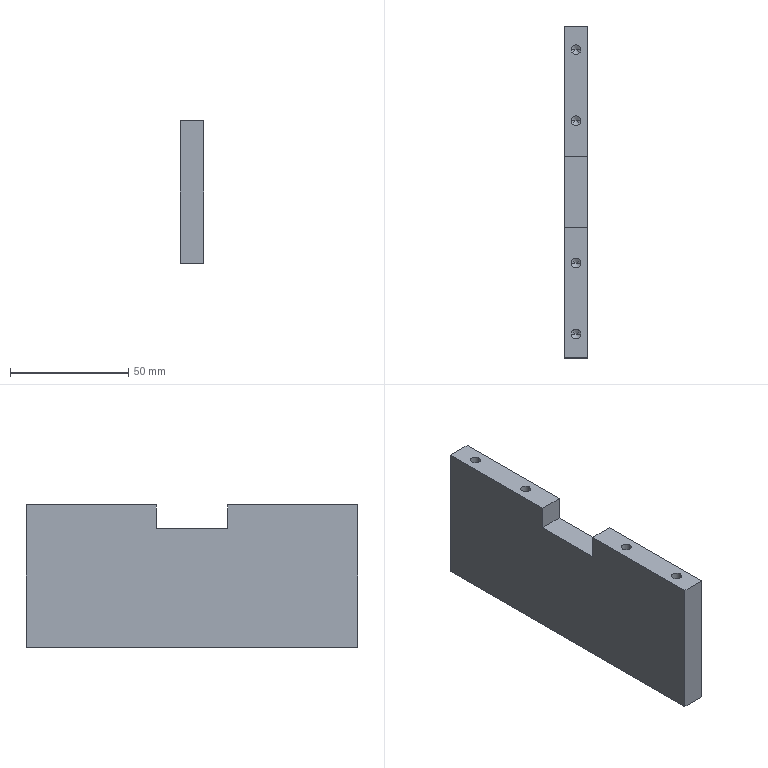Part | SolidWorks | features HoleWzd 2, Cut 1, Extrusion 1, LPattern 1 | 1 solid | 38 faces | box 10 x 140 x 60 mm | volume 79757 mm3 | cylinder 14 | cone 14 | plane 10 | commonest cylinder face diameters 4.2 x14
STEP:
#1=CARTESIAN_POINT('',(2.9,-60.,17.6));
#2=VERTEX_POINT('',#1);
#3=CARTESIAN_POINT('',(7.1,-60.,17.6));
#4=VERTEX_POINT('',#3);
#5=CARTESIAN_POINT('',(5.,-60.,17.6));
#6=DIRECTION('',(0.,0.,1.));
#7=DIRECTION('',(1.,0.,0.));
#8=AXIS2_PLACEMENT_3D('',#5,#6,#7);
#9=CIRCLE('',#8,2.1);
#10=EDGE_CURVE('',#2,#4,#9,.T.);
#11=ORIENTED_EDGE('',*,*,#10,.F.);
#12=CARTESIAN_POINT('',(2.9,-60.,30.));
#13=VERTEX_POINT('',#12);
#14=CARTESIAN_POINT('',(2.9,-60.,30.));
#15=DIRECTION('',(0.,0.,1.));
#16=VECTOR('',#15,1000.);
#17=LINE('',#14,#16);
#18=EDGE_CURVE('',#2,#13,#17,.T.);
#19=ORIENTED_EDGE('',*,*,#18,.T.);
#20=CARTESIAN_POINT('',(7.1,-60.,30.));
#21=VERTEX_POINT('',#20);
#22=CARTESIAN_POINT('',(5.,-60.,30.));
#23=DIRECTION('',(0.,0.,1.));
#24=DIRECTION('',(1.,0.,0.));
#25=AXIS2_PLACEMENT_3D('',#22,#23,#24);
#26=CIRCLE('',#25,2.1);
#27=EDGE_CURVE('',#13,#21,#26,.T.);
#28=ORIENTED_EDGE('',*,*,#27,.T.);
#29=CARTESIAN_POINT('',(7.1,-60.,30.));
#30=DIRECTION('',(0.,0.,1.));
#31=VECTOR('',#30,1000.);
#32=LINE('',#29,#31);
#33=EDGE_CURVE('',#4,#21,#32,.T.);
#34=ORIENTED_EDGE('',*,*,#33,.F.);
#35=EDGE_LOOP('',(#11,#19,#28,#34));
#36=FACE_OUTER_BOUND('',#35,.T.);
#37=CARTESIAN_POINT('',(5.,-60.,30.));
#38=DIRECTION('',(0.,0.,1.));
#39=DIRECTION('',(1.,0.,0.));
#40=AXIS2_PLACEMENT_3D('',#37,#38,#39);
#41=CYLINDRICAL_SURFACE('',#40,2.1);
#42=ADVANCED_FACE('',(#36),#41,.F.);
#43=CARTESIAN_POINT('',(5.,-60.,16.338));
#44=VERTEX_POINT('',#43);
#45=CARTESIAN_POINT('',(7.1,-60.,17.6));
#46=DIRECTION('',(0.8572,0.,0.515));
#47=VECTOR('',#46,1000.);
#48=LINE('',#45,#47);
#49=EDGE_CURVE('',#44,#4,#48,.T.);
#50=ORIENTED_EDGE('',*,*,#49,.F.);
#51=CARTESIAN_POINT('',(2.9,-60.,17.6));
#52=DIRECTION('',(-0.8572,0.,0.515));
#53=VECTOR('',#52,1000.);
#54=LINE('',#51,#53);
#55=EDGE_CURVE('',#44,#2,#54,.T.);
#56=ORIENTED_EDGE('',*,*,#55,.T.);
#57=ORIENTED_EDGE('',*,*,#10,.T.);
#58=EDGE_LOOP('',(#50,#56,#57));
#59=FACE_OUTER_BOUND('',#58,.T.);
#60=CARTESIAN_POINT('',(5.,-60.,17.6));
#61=DIRECTION('',(0.,0.,1.));
#62=DIRECTION('',(1.,0.,0.));
#63=AXIS2_PLACEMENT_3D('',#60,#61,#62);
#64=CONICAL_SURFACE('',#63,2.1,1.03);
#65=ADVANCED_FACE('',(#59),#64,.F.);
#66=CARTESIAN_POINT('',(2.9,-30.,17.6));
#67=VERTEX_POINT('',#66);
#68=CARTESIAN_POINT('',(7.1,-30.,17.6));
#69=VERTEX_POINT('',#68);
#70=CARTESIAN_POINT('',(5.,-30.,17.6));
#71=DIRECTION('',(0.,0.,1.));
#72=DIRECTION('',(1.,0.,0.));
#73=AXIS2_PLACEMENT_3D('',#70,#71,#72);
#74=CIRCLE('',#73,2.1);
#75=EDGE_CURVE('',#67,#69,#74,.T.);
#76=ORIENTED_EDGE('',*,*,#75,.F.);
#77=CARTESIAN_POINT('',(2.9,-30.,30.));
#78=VERTEX_POINT('',#77);
#79=CARTESIAN_POINT('',(2.9,-30.,30.));
#80=DIRECTION('',(0.,0.,1.));
#81=VECTOR('',#80,1000.);
#82=LINE('',#79,#81);
#83=EDGE_CURVE('',#67,#78,#82,.T.);
#84=ORIENTED_EDGE('',*,*,#83,.T.);
#85=CARTESIAN_POINT('',(7.1,-30.,30.));
#86=VERTEX_POINT('',#85);
#87=CARTESIAN_POINT('',(5.,-30.,30.));
#88=DIRECTION('',(0.,0.,1.));
#89=DIRECTION('',(1.,0.,0.));
#90=AXIS2_PLACEMENT_3D('',#87,#88,#89);
#91=CIRCLE('',#90,2.1);
#92=EDGE_CURVE('',#78,#86,#91,.T.);
#93=ORIENTED_EDGE('',*,*,#92,.T.);
#94=CARTESIAN_POINT('',(7.1,-30.,30.));
#95=DIRECTION('',(0.,0.,1.));
#96=VECTOR('',#95,1000.);
#97=LINE('',#94,#96);
#98=EDGE_CURVE('',#69,#86,#97,.T.);
#99=ORIENTED_EDGE('',*,*,#98,.F.);
#100=EDGE_LOOP('',(#76,#84,#93,#99));
#101=FACE_OUTER_BOUND('',#100,.T.);
#102=CARTESIAN_POINT('',(5.,-30.,30.));
#103=DIRECTION('',(0.,0.,1.));
#104=DIRECTION('',(1.,0.,0.));
#105=AXIS2_PLACEMENT_3D('',#102,#103,#104);
#106=CYLINDRICAL_SURFACE('',#105,2.1);
#107=ADVANCED_FACE('',(#101),#106,.F.);
#108=CARTESIAN_POINT('',(5.,-30.,16.338));
#109=VERTEX_POINT('',#108);
#110=CARTESIAN_POINT('',(7.1,-30.,17.6));
#111=DIRECTION('',(0.8572,0.,0.515));
#112=VECTOR('',#111,1000.);
#113=LINE('',#110,#112);
#114=EDGE_CURVE('',#109,#69,#113,.T.);
#115=ORIENTED_EDGE('',*,*,#114,.F.);
#116=CARTESIAN_POINT('',(2.9,-30.,17.6));
#117=DIRECTION('',(-0.8572,0.,0.515));
#118=VECTOR('',#117,1000.);
#119=LINE('',#116,#118);
#120=EDGE_CURVE('',#109,#67,#119,.T.);
#121=ORIENTED_EDGE('',*,*,#120,.T.);
#122=ORIENTED_EDGE('',*,*,#75,.T.);
#123=EDGE_LOOP('',(#115,#121,#122));
#124=FACE_OUTER_BOUND('',#123,.T.);
#125=CARTESIAN_POINT('',(5.,-30.,17.6));
#126=DIRECTION('',(0.,0.,1.));
#127=DIRECTION('',(1.,0.,0.));
#128=AXIS2_PLACEMENT_3D('',#125,#126,#127);
#129=CONICAL_SURFACE('',#128,2.1,1.03);
#130=ADVANCED_FACE('',(#124),#129,.F.);
#131=CARTESIAN_POINT('',(2.9,30.,17.6));
#132=VERTEX_POINT('',#131);
#133=CARTESIAN_POINT('',(7.1,30.,17.6));
#134=VERTEX_POINT('',#133);
#135=CARTESIAN_POINT('',(5.,30.,17.6));
#136=DIRECTION('',(0.,0.,1.));
#137=DIRECTION('',(1.,0.,0.));
#138=AXIS2_PLACEMENT_3D('',#135,#136,#137);
#139=CIRCLE('',#138,2.1);
#140=EDGE_CURVE('',#132,#134,#139,.T.);
#141=ORIENTED_EDGE('',*,*,#140,.F.);
#142=CARTESIAN_POINT('',(2.9,30.,30.));
#143=VERTEX_POINT('',#142);
#144=CARTESIAN_POINT('',(2.9,30.,30.));
#145=DIRECTION('',(0.,0.,1.));
#146=VECTOR('',#145,1000.);
#147=LINE('',#144,#146);
#148=EDGE_CURVE('',#132,#143,#147,.T.);
#149=ORIENTED_EDGE('',*,*,#148,.T.);
#150=CARTESIAN_POINT('',(7.1,30.,30.));
#151=VERTEX_POINT('',#150);
#152=CARTESIAN_POINT('',(5.,30.,30.));
#153=DIRECTION('',(0.,0.,1.));
#154=DIRECTION('',(1.,0.,0.));
#155=AXIS2_PLACEMENT_3D('',#152,#153,#154);
#156=CIRCLE('',#155,2.1);
#157=EDGE_CURVE('',#143,#151,#156,.T.);
#158=ORIENTED_EDGE('',*,*,#157,.T.);
#159=CARTESIAN_POINT('',(7.1,30.,30.));
#160=DIRECTION('',(0.,0.,1.));
#161=VECTOR('',#160,1000.);
#162=LINE('',#159,#161);
#163=EDGE_CURVE('',#134,#151,#162,.T.);
#164=ORIENTED_EDGE('',*,*,#163,.F.);
#165=EDGE_LOOP('',(#141,#149,#158,#164));
#166=FACE_OUTER_BOUND('',#165,.T.);
#167=CARTESIAN_POINT('',(5.,30.,30.));
#168=DIRECTION('',(0.,0.,1.));
#169=DIRECTION('',(1.,0.,0.));
#170=AXIS2_PLACEMENT_3D('',#167,#168,#169);
#171=CYLINDRICAL_SURFACE('',#170,2.1);
#172=ADVANCED_FACE('',(#166),#171,.F.);
#173=CARTESIAN_POINT('',(5.,30.,16.338));
#174=VERTEX_POINT('',#173);
#175=CARTESIAN_POINT('',(7.1,30.,17.6));
#176=DIRECTION('',(0.8572,0.,0.515));
#177=VECTOR('',#176,1000.);
#178=LINE('',#175,#177);
#179=EDGE_CURVE('',#174,#134,#178,.T.);
#180=ORIENTED_EDGE('',*,*,#179,.F.);
#181=CARTESIAN_POINT('',(2.9,30.,17.6));
#182=DIRECTION('',(-0.8572,0.,0.515));
#183=VECTOR('',#182,1000.);
#184=LINE('',#181,#183);
#185=EDGE_CURVE('',#174,#132,#184,.T.);
#186=ORIENTED_EDGE('',*,*,#185,.T.);
#187=ORIENTED_EDGE('',*,*,#140,.T.);
#188=EDGE_LOOP('',(#180,#186,#187));
#189=FACE_OUTER_BOUND('',#188,.T.);
#190=CARTESIAN_POINT('',(5.,30.,17.6));
#191=DIRECTION('',(0.,0.,1.));
#192=DIRECTION('',(1.,0.,0.));
#193=AXIS2_PLACEMENT_3D('',#190,#191,#192);
#194=CONICAL_SURFACE('',#193,2.1,1.03);
#195=ADVANCED_FACE('',(#189),#194,.F.);
#196=CARTESIAN_POINT('',(2.9,60.,17.6));
#197=VERTEX_POINT('',#196);
#198=CARTESIAN_POINT('',(7.1,60.,17.6));
#199=VERTEX_POINT('',#198);
#200=CARTESIAN_POINT('',(5.,60.,17.6));
#201=DIRECTION('',(0.,0.,1.));
#202=DIRECTION('',(1.,0.,0.));
#203=AXIS2_PLACEMENT_3D('',#200,#201,#202);
#204=CIRCLE('',#203,2.1);
#205=EDGE_CURVE('',#197,#199,#204,.T.);
#206=ORIENTED_EDGE('',*,*,#205,.F.);
#207=CARTESIAN_POINT('',(2.9,60.,30.));
#208=VERTEX_POINT('',#207);
#209=CARTESIAN_POINT('',(2.9,60.,30.));
#210=DIRECTION('',(0.,0.,1.));
#211=VECTOR('',#210,1000.);
#212=LINE('',#209,#211);
#213=EDGE_CURVE('',#197,#208,#212,.T.);
#214=ORIENTED_EDGE('',*,*,#213,.T.);
#215=CARTESIAN_POINT('',(7.1,60.,30.));
#216=VERTEX_POINT('',#215);
#217=CARTESIAN_POINT('',(5.,60.,30.));
#218=DIRECTION('',(0.,0.,1.));
#219=DIRECTION('',(1.,0.,0.));
#220=AXIS2_PLACEMENT_3D('',#217,#218,#219);
#221=CIRCLE('',#220,2.1);
#222=EDGE_CURVE('',#208,#216,#221,.T.);
#223=ORIENTED_EDGE('',*,*,#222,.T.);
#224=CARTESIAN_POINT('',(7.1,60.,30.));
#225=DIRECTION('',(0.,0.,1.));
#226=VECTOR('',#225,1000.);
#227=LINE('',#224,#226);
#228=EDGE_CURVE('',#199,#216,#227,.T.);
#229=ORIENTED_EDGE('',*,*,#228,.F.);
#230=EDGE_LOOP('',(#206,#214,#223,#229));
#231=FACE_OUTER_BOUND('',#230,.T.);
#232=CARTESIAN_POINT('',(5.,60.,30.));
#233=DIRECTION('',(0.,0.,1.));
#234=DIRECTION('',(1.,0.,0.));
#235=AXIS2_PLACEMENT_3D('',#232,#233,#234);
#236=CYLINDRICAL_SURFACE('',#235,2.1);
#237=ADVANCED_FACE('',(#231),#236,.F.);
#238=CARTESIAN_POINT('',(5.,60.,16.338));
#239=VERTEX_POINT('',#238);
#240=CARTESIAN_POINT('',(7.1,60.,17.6));
#241=DIRECTION('',(0.8572,0.,0.515));
#242=VECTOR('',#241,1000.);
#243=LINE('',#240,#242);
#244=EDGE_CURVE('',#239,#199,#243,.T.);
#245=ORIENTED_EDGE('',*,*,#244,.F.);
#246=CARTESIAN_POINT('',(2.9,60.,17.6));
#247=DIRECTION('',(-0.8572,0.,0.515));
#248=VECTOR('',#247,1000.);
#249=LINE('',#246,#248);
#250=EDGE_CURVE('',#239,#197,#249,.T.);
#251=ORIENTED_EDGE('',*,*,#250,.T.);
#252=ORIENTED_EDGE('',*,*,#205,.T.);
#253=EDGE_LOOP('',(#245,#251,#252));
#254=FACE_OUTER_BOUND('',#253,.T.);
#255=CARTESIAN_POINT('',(5.,60.,17.6));
#256=DIRECTION('',(0.,0.,1.));
#257=DIRECTION('',(1.,0.,0.));
#258=AXIS2_PLACEMENT_3D('',#255,#256,#257);
#259=CONICAL_SURFACE('',#258,2.1,1.03);
#260=ADVANCED_FACE('',(#254),#259,.F.);
#261=CARTESIAN_POINT('',(5.,-60.,-16.338));
#262=VERTEX_POINT('',#261);
#263=CARTESIAN_POINT('',(2.9,-60.,-17.6));
#264=VERTEX_POINT('',#263);
#265=CARTESIAN_POINT('',(2.9,-60.,-17.6));
#266=DIRECTION('',(-0.8572,0.,-0.515));
#267=VECTOR('',#266,1000.);
#268=LINE('',#265,#267);
#269=EDGE_CURVE('',#262,#264,#268,.T.);
#270=ORIENTED_EDGE('',*,*,#269,.F.);
#271=CARTESIAN_POINT('',(7.1,-60.,-17.6));
#272=VERTEX_POINT('',#271);
#273=CARTESIAN_POINT('',(7.1,-60.,-17.6));
#274=DIRECTION('',(0.8572,0.,-0.515));
#275=VECTOR('',#274,1000.);
#276=LINE('',#273,#275);
#277=EDGE_CURVE('',#262,#272,#276,.T.);
#278=ORIENTED_EDGE('',*,*,#277,.T.);
#279=CARTESIAN_POINT('',(5.,-60.,-17.6));
#280=DIRECTION('',(0.,0.,-1.));
#281=DIRECTION('',(-1.,0.,0.));
#282=AXIS2_PLACEMENT_3D('',#279,#280,#281);
#283=CIRCLE('',#282,2.1);
#284=EDGE_CURVE('',#272,#264,#283,.T.);
#285=ORIENTED_EDGE('',*,*,#284,.T.);
#286=EDGE_LOOP('',(#270,#278,#285));
#287=FACE_OUTER_BOUND('',#286,.T.);
#288=CARTESIAN_POINT('',(5.,-60.,-17.6));
#289=DIRECTION('',(0.,0.,-1.));
#290=DIRECTION('',(-1.,0.,0.));
#291=AXIS2_PLACEMENT_3D('',#288,#289,#290);
#292=CONICAL_SURFACE('',#291,2.1,1.03);
#293=ADVANCED_FACE('',(#287),#292,.F.);
#294=ORIENTED_EDGE('',*,*,#284,.F.);
#295=CARTESIAN_POINT('',(7.1,-60.,-30.));
#296=VERTEX_POINT('',#295);
#297=CARTESIAN_POINT('',(7.1,-60.,-30.));
#298=DIRECTION('',(0.,0.,-1.));
#299=VECTOR('',#298,1000.);
#300=LINE('',#297,#299);
#301=EDGE_CURVE('',#272,#296,#300,.T.);
#302=ORIENTED_EDGE('',*,*,#301,.T.);
#303=CARTESIAN_POINT('',(2.9,-60.,-30.));
#304=VERTEX_POINT('',#303);
#305=CARTESIAN_POINT('',(5.,-60.,-30.));
#306=DIRECTION('',(0.,0.,-1.));
#307=DIRECTION('',(-1.,0.,0.));
#308=AXIS2_PLACEMENT_3D('',#305,#306,#307);
#309=CIRCLE('',#308,2.1);
#310=EDGE_CURVE('',#296,#304,#309,.T.);
#311=ORIENTED_EDGE('',*,*,#310,.T.);
#312=CARTESIAN_POINT('',(2.9,-60.,-30.));
#313=DIRECTION('',(0.,0.,-1.));
#314=VECTOR('',#313,1000.);
#315=LINE('',#312,#314);
#316=EDGE_CURVE('',#264,#304,#315,.T.);
#317=ORIENTED_EDGE('',*,*,#316,.F.);
#318=EDGE_LOOP('',(#294,#302,#311,#317));
#319=FACE_OUTER_BOUND('',#318,.T.);
#320=CARTESIAN_POINT('',(5.,-60.,-30.));
#321=DIRECTION('',(0.,0.,-1.));
#322=DIRECTION('',(-1.,0.,0.));
#323=AXIS2_PLACEMENT_3D('',#320,#321,#322);
#324=CYLINDRICAL_SURFACE('',#323,2.1);
#325=ADVANCED_FACE('',(#319),#324,.F.);
#326=CARTESIAN_POINT('',(7.1,0.,-17.6));
#327=VERTEX_POINT('',#326);
#328=CARTESIAN_POINT('',(2.9,0.,-17.6));
#329=VERTEX_POINT('',#328);
#330=CARTESIAN_POINT('',(5.,0.,-17.6));
#331=DIRECTION('',(0.,0.,-1.));
#332=DIRECTION('',(-1.,0.,0.));
#333=AXIS2_PLACEMENT_3D('',#330,#331,#332);
#334=CIRCLE('',#333,2.1);
#335=EDGE_CURVE('',#327,#329,#334,.T.);
#336=ORIENTED_EDGE('',*,*,#335,.F.);
#337=CARTESIAN_POINT('',(7.1,0.,-30.));
#338=VERTEX_POINT('',#337);
#339=CARTESIAN_POINT('',(7.1,0.,-30.));
#340=DIRECTION('',(0.,0.,-1.));
#341=VECTOR('',#340,1000.);
#342=LINE('',#339,#341);
#343=EDGE_CURVE('',#327,#338,#342,.T.);
#344=ORIENTED_EDGE('',*,*,#343,.T.);
#345=CARTESIAN_POINT('',(2.9,0.,-30.));
#346=VERTEX_POINT('',#345);
#347=CARTESIAN_POINT('',(5.,0.,-30.));
#348=DIRECTION('',(0.,0.,-1.));
#349=DIRECTION('',(-1.,0.,0.));
#350=AXIS2_PLACEMENT_3D('',#347,#348,#349);
#351=CIRCLE('',#350,2.1);
#352=EDGE_CURVE('',#338,#346,#351,.T.);
#353=ORIENTED_EDGE('',*,*,#352,.T.);
#354=CARTESIAN_POINT('',(2.9,0.,-30.));
#355=DIRECTION('',(0.,0.,-1.));
#356=VECTOR('',#355,1000.);
#357=LINE('',#354,#356);
#358=EDGE_CURVE('',#329,#346,#357,.T.);
#359=ORIENTED_EDGE('',*,*,#358,.F.);
#360=EDGE_LOOP('',(#336,#344,#353,#359));
#361=FACE_OUTER_BOUND('',#360,.T.);
#362=CARTESIAN_POINT('',(5.,0.,-30.));
#363=DIRECTION('',(0.,0.,-1.));
#364=DIRECTION('',(-1.,0.,0.));
#365=AXIS2_PLACEMENT_3D('',#362,#363,#364);
#366=CYLINDRICAL_SURFACE('',#365,2.1);
#367=ADVANCED_FACE('',(#361),#366,.F.);
#368=CARTESIAN_POINT('',(5.,0.,-16.338));
#369=VERTEX_POINT('',#368);
#370=CARTESIAN_POINT('',(2.9,0.,-17.6));
#371=DIRECTION('',(-0.8572,0.,-0.515));
#372=VECTOR('',#371,1000.);
#373=LINE('',#370,#372);
#374=EDGE_CURVE('',#369,#329,#373,.T.);
#375=ORIENTED_EDGE('',*,*,#374,.F.);
#376=CARTESIAN_POINT('',(7.1,0.,-17.6));
#377=DIRECTION('',(0.8572,0.,-0.515));
#378=VECTOR('',#377,1000.);
#379=LINE('',#376,#378);
#380=EDGE_CURVE('',#369,#327,#379,.T.);
#381=ORIENTED_EDGE('',*,*,#380,.T.);
#382=ORIENTED_EDGE('',*,*,#335,.T.);
#383=EDGE_LOOP('',(#375,#381,#382));
#384=FACE_OUTER_BOUND('',#383,.T.);
#385=CARTESIAN_POINT('',(5.,0.,-17.6));
#386=DIRECTION('',(0.,0.,-1.));
#387=DIRECTION('',(-1.,0.,0.));
#388=AXIS2_PLACEMENT_3D('',#385,#386,#387);
#389=CONICAL_SURFACE('',#388,2.1,1.03);
#390=ADVANCED_FACE('',(#384),#389,.F.);
#391=CARTESIAN_POINT('',(7.1,60.,-17.6));
#392=VERTEX_POINT('',#391);
#393=CARTESIAN_POINT('',(2.9,60.,-17.6));
#394=VERTEX_POINT('',#393);
#395=CARTESIAN_POINT('',(5.,60.,-17.6));
#396=DIRECTION('',(0.,0.,-1.));
#397=DIRECTION('',(-1.,0.,0.));
#398=AXIS2_PLACEMENT_3D('',#395,#396,#397);
#399=CIRCLE('',#398,2.1);
#400=EDGE_CURVE('',#392,#394,#399,.T.);
#401=ORIENTED_EDGE('',*,*,#400,.F.);
#402=CARTESIAN_POINT('',(7.1,60.,-30.));
#403=VERTEX_POINT('',#402);
#404=CARTESIAN_POINT('',(7.1,60.,-30.));
#405=DIRECTION('',(0.,0.,-1.));
#406=VECTOR('',#405,1000.);
#407=LINE('',#404,#406);
#408=EDGE_CURVE('',#392,#403,#407,.T.);
#409=ORIENTED_EDGE('',*,*,#408,.T.);
#410=CARTESIAN_POINT('',(2.9,60.,-30.));
#411=VERTEX_POINT('',#410);
#412=CARTESIAN_POINT('',(5.,60.,-30.));
#413=DIRECTION('',(0.,0.,-1.));
#414=DIRECTION('',(-1.,0.,0.));
#415=AXIS2_PLACEMENT_3D('',#412,#413,#414);
#416=CIRCLE('',#415,2.1);
#417=EDGE_CURVE('',#403,#411,#416,.T.);
#418=ORIENTED_EDGE('',*,*,#417,.T.);
#419=CARTESIAN_POINT('',(2.9,60.,-30.));
#420=DIRECTION('',(0.,0.,-1.));
#421=VECTOR('',#420,1000.);
#422=LINE('',#419,#421);
#423=EDGE_CURVE('',#394,#411,#422,.T.);
#424=ORIENTED_EDGE('',*,*,#423,.F.);
#425=EDGE_LOOP('',(#401,#409,#418,#424));
#426=FACE_OUTER_BOUND('',#425,.T.);
#427=CARTESIAN_POINT('',(5.,60.,-30.));
#428=DIRECTION('',(0.,0.,-1.));
#429=DIRECTION('',(-1.,0.,0.));
#430=AXIS2_PLACEMENT_3D('',#427,#428,#429);
#431=CYLINDRICAL_SURFACE('',#430,2.1);
#432=ADVANCED_FACE('',(#426),#431,.F.);
#433=CARTESIAN_POINT('',(5.,60.,-16.338));
#434=VERTEX_POINT('',#433);
#435=CARTESIAN_POINT('',(2.9,60.,-17.6));
#436=DIRECTION('',(-0.8572,0.,-0.515));
#437=VECTOR('',#436,1000.);
#438=LINE('',#435,#437);
#439=EDGE_CURVE('',#434,#394,#438,.T.);
#440=ORIENTED_EDGE('',*,*,#439,.F.);
#441=CARTESIAN_POINT('',(7.1,60.,-17.6));
#442=DIRECTION('',(0.8572,0.,-0.515));
#443=VECTOR('',#442,1000.);
#444=LINE('',#441,#443);
#445=EDGE_CURVE('',#434,#392,#444,.T.);
#446=ORIENTED_EDGE('',*,*,#445,.T.);
#447=ORIENTED_EDGE('',*,*,#400,.T.);
#448=EDGE_LOOP('',(#440,#446,#447));
#449=FACE_OUTER_BOUND('',#448,.T.);
#450=CARTESIAN_POINT('',(5.,60.,-17.6));
#451=DIRECTION('',(0.,0.,-1.));
#452=DIRECTION('',(-1.,0.,0.));
#453=AXIS2_PLACEMENT_3D('',#450,#451,#452);
#454=CONICAL_SURFACE('',#453,2.1,1.03);
#455=ADVANCED_FACE('',(#449),#454,.F.);
#456=CARTESIAN_POINT('',(5.,-60.,30.));
#457=DIRECTION('',(0.,0.,1.));
#458=DIRECTION('',(1.,0.,0.));
#459=AXIS2_PLACEMENT_3D('',#456,#457,#458);
#460=CIRCLE('',#459,2.1);
#461=EDGE_CURVE('',#21,#13,#460,.T.);
#462=ORIENTED_EDGE('',*,*,#461,.F.);
#463=ORIENTED_EDGE('',*,*,#27,.F.);
#464=EDGE_LOOP('',(#462,#463));
#465=FACE_BOUND('',#464,.T.);
#466=CARTESIAN_POINT('',(5.,-30.,30.));
#467=DIRECTION('',(0.,0.,1.));
#468=DIRECTION('',(1.,0.,0.));
#469=AXIS2_PLACEMENT_3D('',#466,#467,#468);
#470=CIRCLE('',#469,2.1);
#471=EDGE_CURVE('',#86,#78,#470,.T.);
#472=ORIENTED_EDGE('',*,*,#471,.F.);
#473=ORIENTED_EDGE('',*,*,#92,.F.);
#474=EDGE_LOOP('',(#472,#473));
#475=FACE_BOUND('',#474,.T.);
#476=CARTESIAN_POINT('',(10.,-15.,30.));
#477=VERTEX_POINT('',#476);
#478=CARTESIAN_POINT('',(10.,-70.,30.));
#479=VERTEX_POINT('',#478);
#480=CARTESIAN_POINT('',(10.,-70.,30.));
#481=DIRECTION('',(0.,-1.,0.));
#482=VECTOR('',#481,1000.);
#483=LINE('',#480,#482);
#484=EDGE_CURVE('',#477,#479,#483,.T.);
#485=ORIENTED_EDGE('',*,*,#484,.F.);
#486=CARTESIAN_POINT('',(0.,-15.,30.));
#487=VERTEX_POINT('',#486);
#488=CARTESIAN_POINT('',(10.,-15.,30.));
#489=DIRECTION('',(-1.,0.,0.));
#490=VECTOR('',#489,1000.);
#491=LINE('',#488,#490);
#492=EDGE_CURVE('',#477,#487,#491,.T.);
#493=ORIENTED_EDGE('',*,*,#492,.T.);
#494=CARTESIAN_POINT('',(0.,-70.,30.));
#495=VERTEX_POINT('',#494);
#496=CARTESIAN_POINT('',(0.,-70.,30.));
#497=DIRECTION('',(0.,-1.,0.));
#498=VECTOR('',#497,1000.);
#499=LINE('',#496,#498);
#500=EDGE_CURVE('',#487,#495,#499,.T.);
#501=ORIENTED_EDGE('',*,*,#500,.T.);
#502=CARTESIAN_POINT('',(10.,-70.,30.));
#503=DIRECTION('',(-1.,0.,0.));
#504=VECTOR('',#503,1000.);
#505=LINE('',#502,#504);
#506=EDGE_CURVE('',#479,#495,#505,.T.);
#507=ORIENTED_EDGE('',*,*,#506,.F.);
#508=EDGE_LOOP('',(#485,#493,#501,#507));
#509=FACE_OUTER_BOUND('',#508,.T.);
#510=CARTESIAN_POINT('',(10.,-70.,30.));
#511=DIRECTION('',(0.,0.,-1.));
#512=DIRECTION('',(-1.,0.,0.));
#513=AXIS2_PLACEMENT_3D('',#510,#511,#512);
#514=PLANE('',#513);
#515=ADVANCED_FACE('',(#465,#475,#509),#514,.F.);
#516=CARTESIAN_POINT('',(5.,0.,-30.));
#517=DIRECTION('',(0.,0.,-1.));
#518=DIRECTION('',(-1.,0.,0.));
#519=AXIS2_PLACEMENT_3D('',#516,#517,#518);
#520=CIRCLE('',#519,2.1);
#521=EDGE_CURVE('',#346,#338,#520,.T.);
#522=ORIENTED_EDGE('',*,*,#521,.F.);
#523=ORIENTED_EDGE('',*,*,#352,.F.);
#524=EDGE_LOOP('',(#522,#523));
#525=FACE_BOUND('',#524,.T.);
#526=CARTESIAN_POINT('',(5.,60.,-30.));
#527=DIRECTION('',(0.,0.,-1.));
#528=DIRECTION('',(-1.,0.,0.));
#529=AXIS2_PLACEMENT_3D('',#526,#527,#528);
#530=CIRCLE('',#529,2.1);
#531=EDGE_CURVE('',#411,#403,#530,.T.);
#532=ORIENTED_EDGE('',*,*,#531,.F.);
#533=ORIENTED_EDGE('',*,*,#417,.F.);
#534=EDGE_LOOP('',(#532,#533));
#535=FACE_BOUND('',#534,.T.);
#536=CARTESIAN_POINT('',(0.,-70.,-30.));
#537=VERTEX_POINT('',#536);
#538=CARTESIAN_POINT('',(0.,70.,-30.));
#539=VERTEX_POINT('',#538);
#540=CARTESIAN_POINT('',(0.,-70.,-30.));
#541=DIRECTION('',(0.,1.,0.));
#542=VECTOR('',#541,1000.);
#543=LINE('',#540,#542);
#544=EDGE_CURVE('',#537,#539,#543,.T.);
#545=ORIENTED_EDGE('',*,*,#544,.T.);
#546=CARTESIAN_POINT('',(10.,70.,-30.));
#547=VERTEX_POINT('',#546);
#548=CARTESIAN_POINT('',(10.,70.,-30.));
#549=DIRECTION('',(-1.,0.,0.));
#550=VECTOR('',#549,1000.);
#551=LINE('',#548,#550);
#552=EDGE_CURVE('',#547,#539,#551,.T.);
#553=ORIENTED_EDGE('',*,*,#552,.F.);
#554=CARTESIAN_POINT('',(10.,-70.,-30.));
#555=VERTEX_POINT('',#554);
#556=CARTESIAN_POINT('',(10.,-70.,-30.));
#557=DIRECTION('',(0.,1.,0.));
#558=VECTOR('',#557,1000.);
#559=LINE('',#556,#558);
#560=EDGE_CURVE('',#555,#547,#559,.T.);
#561=ORIENTED_EDGE('',*,*,#560,.F.);
#562=CARTESIAN_POINT('',(10.,-70.,-30.));
#563=DIRECTION('',(-1.,0.,0.));
#564=VECTOR('',#563,1000.);
#565=LINE('',#562,#564);
#566=EDGE_CURVE('',#555,#537,#565,.T.);
#567=ORIENTED_EDGE('',*,*,#566,.T.);
#568=EDGE_LOOP('',(#545,#553,#561,#567));
#569=FACE_OUTER_BOUND('',#568,.T.);
#570=CARTESIAN_POINT('',(5.,-60.,-30.));
#571=DIRECTION('',(0.,0.,-1.));
#572=DIRECTION('',(-1.,0.,0.));
#573=AXIS2_PLACEMENT_3D('',#570,#571,#572);
#574=CIRCLE('',#573,2.1);
#575=EDGE_CURVE('',#304,#296,#574,.T.);
#576=ORIENTED_EDGE('',*,*,#575,.F.);
#577=ORIENTED_EDGE('',*,*,#310,.F.);
#578=EDGE_LOOP('',(#576,#577));
#579=FACE_BOUND('',#578,.T.);
#580=CARTESIAN_POINT('',(10.,-70.,-30.));
#581=DIRECTION('',(0.,0.,1.));
#582=DIRECTION('',(1.,0.,0.));
#583=AXIS2_PLACEMENT_3D('',#580,#581,#582);
#584=PLANE('',#583);
#585=ADVANCED_FACE('',(#525,#535,#569,#579),#584,.F.);
#586=CARTESIAN_POINT('',(0.,70.,30.));
#587=VERTEX_POINT('',#586);
#588=CARTESIAN_POINT('',(0.,70.,30.));
#589=DIRECTION('',(0.,0.,1.));
#590=VECTOR('',#589,1000.);
#591=LINE('',#588,#590);
#592=EDGE_CURVE('',#539,#587,#591,.T.);
#593=ORIENTED_EDGE('',*,*,#592,.T.);
#594=CARTESIAN_POINT('',(10.,70.,30.));
#595=VERTEX_POINT('',#594);
#596=CARTESIAN_POINT('',(10.,70.,30.));
#597=DIRECTION('',(-1.,0.,0.));
#598=VECTOR('',#597,1000.);
#599=LINE('',#596,#598);
#600=EDGE_CURVE('',#595,#587,#599,.T.);
#601=ORIENTED_EDGE('',*,*,#600,.F.);
#602=CARTESIAN_POINT('',(10.,70.,30.));
#603=DIRECTION('',(0.,0.,1.));
#604=VECTOR('',#603,1000.);
#605=LINE('',#602,#604);
#606=EDGE_CURVE('',#547,#595,#605,.T.);
#607=ORIENTED_EDGE('',*,*,#606,.F.);
#608=ORIENTED_EDGE('',*,*,#552,.T.);
#609=EDGE_LOOP('',(#593,#601,#607,#608));
#610=FACE_OUTER_BOUND('',#609,.T.);
#611=CARTESIAN_POINT('',(10.,70.,30.));
#612=DIRECTION('',(0.,-1.,0.));
#613=DIRECTION('',(0.,0.,-1.));
#614=AXIS2_PLACEMENT_3D('',#611,#612,#613);
#615=PLANE('',#614);
#616=ADVANCED_FACE('',(#610),#615,.F.);
#617=CARTESIAN_POINT('',(5.,30.,30.));
#618=DIRECTION('',(0.,0.,1.));
#619=DIRECTION('',(1.,0.,0.));
#620=AXIS2_PLACEMENT_3D('',#617,#618,#619);
#621=CIRCLE('',#620,2.1);
#622=EDGE_CURVE('',#151,#143,#621,.T.);
#623=ORIENTED_EDGE('',*,*,#622,.F.);
#624=ORIENTED_EDGE('',*,*,#157,.F.);
#625=EDGE_LOOP('',(#623,#624));
#626=FACE_BOUND('',#625,.T.);
#627=CARTESIAN_POINT('',(5.,60.,30.));
#628=DIRECTION('',(0.,0.,1.));
#629=DIRECTION('',(1.,0.,0.));
#630=AXIS2_PLACEMENT_3D('',#627,#628,#629);
#631=CIRCLE('',#630,2.1);
#632=EDGE_CURVE('',#216,#208,#631,.T.);
#633=ORIENTED_EDGE('',*,*,#632,.F.);
#634=ORIENTED_EDGE('',*,*,#222,.F.);
#635=EDGE_LOOP('',(#633,#634));
#636=FACE_BOUND('',#635,.T.);
#637=CARTESIAN_POINT('',(0.,15.,30.));
#638=VERTEX_POINT('',#637);
#639=CARTESIAN_POINT('',(0.,-70.,30.));
#640=DIRECTION('',(0.,-1.,0.));
#641=VECTOR('',#640,1000.);
#642=LINE('',#639,#641);
#643=EDGE_CURVE('',#587,#638,#642,.T.);
#644=ORIENTED_EDGE('',*,*,#643,.T.);
#645=CARTESIAN_POINT('',(10.,15.,30.));
#646=VERTEX_POINT('',#645);
#647=CARTESIAN_POINT('',(10.,15.,30.));
#648=DIRECTION('',(-1.,0.,0.));
#649=VECTOR('',#648,1000.);
#650=LINE('',#647,#649);
#651=EDGE_CURVE('',#646,#638,#650,.T.);
#652=ORIENTED_EDGE('',*,*,#651,.F.);
#653=CARTESIAN_POINT('',(10.,-70.,30.));
#654=DIRECTION('',(0.,-1.,0.));
#655=VECTOR('',#654,1000.);
#656=LINE('',#653,#655);
#657=EDGE_CURVE('',#595,#646,#656,.T.);
#658=ORIENTED_EDGE('',*,*,#657,.F.);
#659=ORIENTED_EDGE('',*,*,#600,.T.);
#660=EDGE_LOOP('',(#644,#652,#658,#659));
#661=FACE_OUTER_BOUND('',#660,.T.);
#662=CARTESIAN_POINT('',(10.,-70.,30.));
#663=DIRECTION('',(0.,0.,-1.));
#664=DIRECTION('',(-1.,0.,0.));
#665=AXIS2_PLACEMENT_3D('',#662,#663,#664);
#666=PLANE('',#665);
#667=ADVANCED_FACE('',(#626,#636,#661),#666,.F.);
#668=CARTESIAN_POINT('',(0.,-70.,30.));
#669=DIRECTION('',(0.,0.,-1.));
#670=VECTOR('',#669,1000.);
#671=LINE('',#668,#670);
#672=EDGE_CURVE('',#495,#537,#671,.T.);
#673=ORIENTED_EDGE('',*,*,#672,.T.);
#674=ORIENTED_EDGE('',*,*,#566,.F.);
#675=CARTESIAN_POINT('',(10.,-70.,30.));
#676=DIRECTION('',(0.,0.,-1.));
#677=VECTOR('',#676,1000.);
#678=LINE('',#675,#677);
#679=EDGE_CURVE('',#479,#555,#678,.T.);
#680=ORIENTED_EDGE('',*,*,#679,.F.);
#681=ORIENTED_EDGE('',*,*,#506,.T.);
#682=EDGE_LOOP('',(#673,#674,#680,#681));
#683=FACE_OUTER_BOUND('',#682,.T.);
#684=CARTESIAN_POINT('',(10.,-70.,30.));
#685=DIRECTION('',(0.,1.,0.));
#686=DIRECTION('',(0.,0.,1.));
#687=AXIS2_PLACEMENT_3D('',#684,#685,#686);
#688=PLANE('',#687);
#689=ADVANCED_FACE('',(#683),#688,.F.);
#690=CARTESIAN_POINT('',(10.,15.,20.));
#691=VERTEX_POINT('',#690);
#692=CARTESIAN_POINT('',(10.,-15.,20.));
#693=VERTEX_POINT('',#692);
#694=CARTESIAN_POINT('',(10.,-15.,20.));
#695=DIRECTION('',(0.,-1.,0.));
#696=VECTOR('',#695,1000.);
#697=LINE('',#694,#696);
#698=EDGE_CURVE('',#691,#693,#697,.T.);
#699=ORIENTED_EDGE('',*,*,#698,.T.);
#700=CARTESIAN_POINT('',(10.,-15.,30.));
#701=DIRECTION('',(0.,0.,1.));
#702=VECTOR('',#701,1000.);
#703=LINE('',#700,#702);
#704=EDGE_CURVE('',#693,#477,#703,.T.);
#705=ORIENTED_EDGE('',*,*,#704,.T.);
#706=ORIENTED_EDGE('',*,*,#484,.T.);
#707=ORIENTED_EDGE('',*,*,#679,.T.);
#708=ORIENTED_EDGE('',*,*,#560,.T.);
#709=ORIENTED_EDGE('',*,*,#606,.T.);
#710=ORIENTED_EDGE('',*,*,#657,.T.);
#711=CARTESIAN_POINT('',(10.,15.,30.));
#712=DIRECTION('',(0.,0.,-1.));
#713=VECTOR('',#712,1000.);
#714=LINE('',#711,#713);
#715=EDGE_CURVE('',#646,#691,#714,.T.);
#716=ORIENTED_EDGE('',*,*,#715,.T.);
#717=EDGE_LOOP('',(#699,#705,#706,#707,#708,#709,#710,#716));
#718=FACE_OUTER_BOUND('',#717,.T.);
#719=CARTESIAN_POINT('',(10.,70.,-30.));
#720=DIRECTION('',(-1.,0.,0.));
#721=DIRECTION('',(0.,0.,1.));
#722=AXIS2_PLACEMENT_3D('',#719,#720,#721);
#723=PLANE('',#722);
#724=ADVANCED_FACE('',(#718),#723,.F.);
#725=CARTESIAN_POINT('',(0.,-15.,20.));
#726=VERTEX_POINT('',#725);
#727=CARTESIAN_POINT('',(0.,-15.,30.));
#728=DIRECTION('',(0.,0.,1.));
#729=VECTOR('',#728,1000.);
#730=LINE('',#727,#729);
#731=EDGE_CURVE('',#726,#487,#730,.T.);
#732=ORIENTED_EDGE('',*,*,#731,.F.);
#733=CARTESIAN_POINT('',(0.,15.,20.));
#734=VERTEX_POINT('',#733);
#735=CARTESIAN_POINT('',(0.,-15.,20.));
#736=DIRECTION('',(0.,-1.,0.));
#737=VECTOR('',#736,1000.);
#738=LINE('',#735,#737);
#739=EDGE_CURVE('',#734,#726,#738,.T.);
#740=ORIENTED_EDGE('',*,*,#739,.F.);
#741=CARTESIAN_POINT('',(0.,15.,30.));
#742=DIRECTION('',(0.,0.,-1.));
#743=VECTOR('',#742,1000.);
#744=LINE('',#741,#743);
#745=EDGE_CURVE('',#638,#734,#744,.T.);
#746=ORIENTED_EDGE('',*,*,#745,.F.);
#747=ORIENTED_EDGE('',*,*,#643,.F.);
#748=ORIENTED_EDGE('',*,*,#592,.F.);
#749=ORIENTED_EDGE('',*,*,#544,.F.);
#750=ORIENTED_EDGE('',*,*,#672,.F.);
#751=ORIENTED_EDGE('',*,*,#500,.F.);
#752=EDGE_LOOP('',(#732,#740,#746,#747,#748,#749,#750,#751));
#753=FACE_OUTER_BOUND('',#752,.T.);
#754=CARTESIAN_POINT('',(0.,70.,-30.));
#755=DIRECTION('',(-1.,0.,0.));
#756=DIRECTION('',(0.,0.,1.));
#757=AXIS2_PLACEMENT_3D('',#754,#755,#756);
#758=PLANE('',#757);
#759=ADVANCED_FACE('',(#753),#758,.T.);
#760=ORIENTED_EDGE('',*,*,#731,.T.);
#761=ORIENTED_EDGE('',*,*,#492,.F.);
#762=ORIENTED_EDGE('',*,*,#704,.F.);
#763=CARTESIAN_POINT('',(10.,-15.,20.));
#764=DIRECTION('',(-1.,0.,0.));
#765=VECTOR('',#764,1000.);
#766=LINE('',#763,#765);
#767=EDGE_CURVE('',#693,#726,#766,.T.);
#768=ORIENTED_EDGE('',*,*,#767,.T.);
#769=EDGE_LOOP('',(#760,#761,#762,#768));
#770=FACE_OUTER_BOUND('',#769,.T.);
#771=CARTESIAN_POINT('',(10.,-15.,30.));
#772=DIRECTION('',(0.,-1.,0.));
#773=DIRECTION('',(0.,0.,-1.));
#774=AXIS2_PLACEMENT_3D('',#771,#772,#773);
#775=PLANE('',#774);
#776=ADVANCED_FACE('',(#770),#775,.F.);
#777=ORIENTED_EDGE('',*,*,#739,.T.);
#778=ORIENTED_EDGE('',*,*,#767,.F.);
#779=ORIENTED_EDGE('',*,*,#698,.F.);
#780=CARTESIAN_POINT('',(10.,15.,20.));
#781=DIRECTION('',(-1.,0.,0.));
#782=VECTOR('',#781,1000.);
#783=LINE('',#780,#782);
#784=EDGE_CURVE('',#691,#734,#783,.T.);
#785=ORIENTED_EDGE('',*,*,#784,.T.);
#786=EDGE_LOOP('',(#777,#778,#779,#785));
#787=FACE_OUTER_BOUND('',#786,.T.);
#788=CARTESIAN_POINT('',(10.,-15.,20.));
#789=DIRECTION('',(0.,0.,-1.));
#790=DIRECTION('',(-1.,0.,0.));
#791=AXIS2_PLACEMENT_3D('',#788,#789,#790);
#792=PLANE('',#791);
#793=ADVANCED_FACE('',(#787),#792,.F.);
#794=ORIENTED_EDGE('',*,*,#745,.T.);
#795=ORIENTED_EDGE('',*,*,#784,.F.);
#796=ORIENTED_EDGE('',*,*,#715,.F.);
#797=ORIENTED_EDGE('',*,*,#651,.T.);
#798=EDGE_LOOP('',(#794,#795,#796,#797));
#799=FACE_OUTER_BOUND('',#798,.T.);
#800=CARTESIAN_POINT('',(10.,15.,30.));
#801=DIRECTION('',(0.,1.,0.));
#802=DIRECTION('',(0.,0.,1.));
#803=AXIS2_PLACEMENT_3D('',#800,#801,#802);
#804=PLANE('',#803);
#805=ADVANCED_FACE('',(#799),#804,.F.);
#806=ORIENTED_EDGE('',*,*,#445,.F.);
#807=ORIENTED_EDGE('',*,*,#439,.T.);
#808=CARTESIAN_POINT('',(5.,60.,-17.6));
#809=DIRECTION('',(0.,0.,-1.));
#810=DIRECTION('',(-1.,0.,0.));
#811=AXIS2_PLACEMENT_3D('',#808,#809,#810);
#812=CIRCLE('',#811,2.1);
#813=EDGE_CURVE('',#394,#392,#812,.T.);
#814=ORIENTED_EDGE('',*,*,#813,.T.);
#815=EDGE_LOOP('',(#806,#807,#814));
#816=FACE_OUTER_BOUND('',#815,.T.);
#817=CARTESIAN_POINT('',(5.,60.,-17.6));
#818=DIRECTION('',(0.,0.,-1.));
#819=DIRECTION('',(-1.,0.,0.));
#820=AXIS2_PLACEMENT_3D('',#817,#818,#819);
#821=CONICAL_SURFACE('',#820,2.1,1.03);
#822=ADVANCED_FACE('',(#816),#821,.F.);
#823=ORIENTED_EDGE('',*,*,#408,.F.);
#824=ORIENTED_EDGE('',*,*,#813,.F.);
#825=ORIENTED_EDGE('',*,*,#423,.T.);
#826=ORIENTED_EDGE('',*,*,#531,.T.);
#827=EDGE_LOOP('',(#823,#824,#825,#826));
#828=FACE_OUTER_BOUND('',#827,.T.);
#829=CARTESIAN_POINT('',(5.,60.,-30.));
#830=DIRECTION('',(0.,0.,-1.));
#831=DIRECTION('',(-1.,0.,0.));
#832=AXIS2_PLACEMENT_3D('',#829,#830,#831);
#833=CYLINDRICAL_SURFACE('',#832,2.1);
#834=ADVANCED_FACE('',(#828),#833,.F.);
#835=ORIENTED_EDGE('',*,*,#343,.F.);
#836=CARTESIAN_POINT('',(5.,0.,-17.6));
#837=DIRECTION('',(0.,0.,-1.));
#838=DIRECTION('',(-1.,0.,0.));
#839=AXIS2_PLACEMENT_3D('',#836,#837,#838);
#840=CIRCLE('',#839,2.1);
#841=EDGE_CURVE('',#329,#327,#840,.T.);
#842=ORIENTED_EDGE('',*,*,#841,.F.);
#843=ORIENTED_EDGE('',*,*,#358,.T.);
#844=ORIENTED_EDGE('',*,*,#521,.T.);
#845=EDGE_LOOP('',(#835,#842,#843,#844));
#846=FACE_OUTER_BOUND('',#845,.T.);
#847=CARTESIAN_POINT('',(5.,0.,-30.));
#848=DIRECTION('',(0.,0.,-1.));
#849=DIRECTION('',(-1.,0.,0.));
#850=AXIS2_PLACEMENT_3D('',#847,#848,#849);
#851=CYLINDRICAL_SURFACE('',#850,2.1);
#852=ADVANCED_FACE('',(#846),#851,.F.);
#853=ORIENTED_EDGE('',*,*,#380,.F.);
#854=ORIENTED_EDGE('',*,*,#374,.T.);
#855=ORIENTED_EDGE('',*,*,#841,.T.);
#856=EDGE_LOOP('',(#853,#854,#855));
#857=FACE_OUTER_BOUND('',#856,.T.);
#858=CARTESIAN_POINT('',(5.,0.,-17.6));
#859=DIRECTION('',(0.,0.,-1.));
#860=DIRECTION('',(-1.,0.,0.));
#861=AXIS2_PLACEMENT_3D('',#858,#859,#860);
#862=CONICAL_SURFACE('',#861,2.1,1.03);
#863=ADVANCED_FACE('',(#857),#862,.F.);
#864=ORIENTED_EDGE('',*,*,#301,.F.);
#865=CARTESIAN_POINT('',(5.,-60.,-17.6));
#866=DIRECTION('',(0.,0.,-1.));
#867=DIRECTION('',(-1.,0.,0.));
#868=AXIS2_PLACEMENT_3D('',#865,#866,#867);
#869=CIRCLE('',#868,2.1);
#870=EDGE_CURVE('',#264,#272,#869,.T.);
#871=ORIENTED_EDGE('',*,*,#870,.F.);
#872=ORIENTED_EDGE('',*,*,#316,.T.);
#873=ORIENTED_EDGE('',*,*,#575,.T.);
#874=EDGE_LOOP('',(#864,#871,#872,#873));
#875=FACE_OUTER_BOUND('',#874,.T.);
#876=CARTESIAN_POINT('',(5.,-60.,-30.));
#877=DIRECTION('',(0.,0.,-1.));
#878=DIRECTION('',(-1.,0.,0.));
#879=AXIS2_PLACEMENT_3D('',#876,#877,#878);
#880=CYLINDRICAL_SURFACE('',#879,2.1);
#881=ADVANCED_FACE('',(#875),#880,.F.);
#882=ORIENTED_EDGE('',*,*,#277,.F.);
#883=ORIENTED_EDGE('',*,*,#269,.T.);
#884=ORIENTED_EDGE('',*,*,#870,.T.);
#885=EDGE_LOOP('',(#882,#883,#884));
#886=FACE_OUTER_BOUND('',#885,.T.);
#887=CARTESIAN_POINT('',(5.,-60.,-17.6));
#888=DIRECTION('',(0.,0.,-1.));
#889=DIRECTION('',(-1.,0.,0.));
#890=AXIS2_PLACEMENT_3D('',#887,#888,#889);
#891=CONICAL_SURFACE('',#890,2.1,1.03);
#892=ADVANCED_FACE('',(#886),#891,.F.);
#893=ORIENTED_EDGE('',*,*,#250,.F.);
#894=ORIENTED_EDGE('',*,*,#244,.T.);
#895=CARTESIAN_POINT('',(5.,60.,17.6));
#896=DIRECTION('',(0.,0.,1.));
#897=DIRECTION('',(1.,0.,0.));
#898=AXIS2_PLACEMENT_3D('',#895,#896,#897);
#899=CIRCLE('',#898,2.1);
#900=EDGE_CURVE('',#199,#197,#899,.T.);
#901=ORIENTED_EDGE('',*,*,#900,.T.);
#902=EDGE_LOOP('',(#893,#894,#901));
#903=FACE_OUTER_BOUND('',#902,.T.);
#904=CARTESIAN_POINT('',(5.,60.,17.6));
#905=DIRECTION('',(0.,0.,1.));
#906=DIRECTION('',(1.,0.,0.));
#907=AXIS2_PLACEMENT_3D('',#904,#905,#906);
#908=CONICAL_SURFACE('',#907,2.1,1.03);
#909=ADVANCED_FACE('',(#903),#908,.F.);
#910=ORIENTED_EDGE('',*,*,#213,.F.);
#911=ORIENTED_EDGE('',*,*,#900,.F.);
#912=ORIENTED_EDGE('',*,*,#228,.T.);
#913=ORIENTED_EDGE('',*,*,#632,.T.);
#914=EDGE_LOOP('',(#910,#911,#912,#913));
#915=FACE_OUTER_BOUND('',#914,.T.);
#916=CARTESIAN_POINT('',(5.,60.,30.));
#917=DIRECTION('',(0.,0.,1.));
#918=DIRECTION('',(1.,0.,0.));
#919=AXIS2_PLACEMENT_3D('',#916,#917,#918);
#920=CYLINDRICAL_SURFACE('',#919,2.1);
#921=ADVANCED_FACE('',(#915),#920,.F.);
#922=ORIENTED_EDGE('',*,*,#185,.F.);
#923=ORIENTED_EDGE('',*,*,#179,.T.);
#924=CARTESIAN_POINT('',(5.,30.,17.6));
#925=DIRECTION('',(0.,0.,1.));
#926=DIRECTION('',(1.,0.,0.));
#927=AXIS2_PLACEMENT_3D('',#924,#925,#926);
#928=CIRCLE('',#927,2.1);
#929=EDGE_CURVE('',#134,#132,#928,.T.);
#930=ORIENTED_EDGE('',*,*,#929,.T.);
#931=EDGE_LOOP('',(#922,#923,#930));
#932=FACE_OUTER_BOUND('',#931,.T.);
#933=CARTESIAN_POINT('',(5.,30.,17.6));
#934=DIRECTION('',(0.,0.,1.));
#935=DIRECTION('',(1.,0.,0.));
#936=AXIS2_PLACEMENT_3D('',#933,#934,#935);
#937=CONICAL_SURFACE('',#936,2.1,1.03);
#938=ADVANCED_FACE('',(#932),#937,.F.);
#939=ORIENTED_EDGE('',*,*,#148,.F.);
#940=ORIENTED_EDGE('',*,*,#929,.F.);
#941=ORIENTED_EDGE('',*,*,#163,.T.);
#942=ORIENTED_EDGE('',*,*,#622,.T.);
#943=EDGE_LOOP('',(#939,#940,#941,#942));
#944=FACE_OUTER_BOUND('',#943,.T.);
#945=CARTESIAN_POINT('',(5.,30.,30.));
#946=DIRECTION('',(0.,0.,1.));
#947=DIRECTION('',(1.,0.,0.));
#948=AXIS2_PLACEMENT_3D('',#945,#946,#947);
#949=CYLINDRICAL_SURFACE('',#948,2.1);
#950=ADVANCED_FACE('',(#944),#949,.F.);
#951=ORIENTED_EDGE('',*,*,#120,.F.);
#952=ORIENTED_EDGE('',*,*,#114,.T.);
#953=CARTESIAN_POINT('',(5.,-30.,17.6));
#954=DIRECTION('',(0.,0.,1.));
#955=DIRECTION('',(1.,0.,0.));
#956=AXIS2_PLACEMENT_3D('',#953,#954,#955);
#957=CIRCLE('',#956,2.1);
#958=EDGE_CURVE('',#69,#67,#957,.T.);
#959=ORIENTED_EDGE('',*,*,#958,.T.);
#960=EDGE_LOOP('',(#951,#952,#959));
#961=FACE_OUTER_BOUND('',#960,.T.);
#962=CARTESIAN_POINT('',(5.,-30.,17.6));
#963=DIRECTION('',(0.,0.,1.));
#964=DIRECTION('',(1.,0.,0.));
#965=AXIS2_PLACEMENT_3D('',#962,#963,#964);
#966=CONICAL_SURFACE('',#965,2.1,1.03);
#967=ADVANCED_FACE('',(#961),#966,.F.);
#968=ORIENTED_EDGE('',*,*,#83,.F.);
#969=ORIENTED_EDGE('',*,*,#958,.F.);
#970=ORIENTED_EDGE('',*,*,#98,.T.);
#971=ORIENTED_EDGE('',*,*,#471,.T.);
#972=EDGE_LOOP('',(#968,#969,#970,#971));
#973=FACE_OUTER_BOUND('',#972,.T.);
#974=CARTESIAN_POINT('',(5.,-30.,30.));
#975=DIRECTION('',(0.,0.,1.));
#976=DIRECTION('',(1.,0.,0.));
#977=AXIS2_PLACEMENT_3D('',#974,#975,#976);
#978=CYLINDRICAL_SURFACE('',#977,2.1);
#979=ADVANCED_FACE('',(#973),#978,.F.);
#980=ORIENTED_EDGE('',*,*,#55,.F.);
#981=ORIENTED_EDGE('',*,*,#49,.T.);
#982=CARTESIAN_POINT('',(5.,-60.,17.6));
#983=DIRECTION('',(0.,0.,1.));
#984=DIRECTION('',(1.,0.,0.));
#985=AXIS2_PLACEMENT_3D('',#982,#983,#984);
#986=CIRCLE('',#985,2.1);
#987=EDGE_CURVE('',#4,#2,#986,.T.);
#988=ORIENTED_EDGE('',*,*,#987,.T.);
#989=EDGE_LOOP('',(#980,#981,#988));
#990=FACE_OUTER_BOUND('',#989,.T.);
#991=CARTESIAN_POINT('',(5.,-60.,17.6));
#992=DIRECTION('',(0.,0.,1.));
#993=DIRECTION('',(1.,0.,0.));
#994=AXIS2_PLACEMENT_3D('',#991,#992,#993);
#995=CONICAL_SURFACE('',#994,2.1,1.03);
#996=ADVANCED_FACE('',(#990),#995,.F.);
#997=ORIENTED_EDGE('',*,*,#18,.F.);
#998=ORIENTED_EDGE('',*,*,#987,.F.);
#999=ORIENTED_EDGE('',*,*,#33,.T.);
#1000=ORIENTED_EDGE('',*,*,#461,.T.);
#1001=EDGE_LOOP('',(#997,#998,#999,#1000));
#1002=FACE_OUTER_BOUND('',#1001,.T.);
#1003=CARTESIAN_POINT('',(5.,-60.,30.));
#1004=DIRECTION('',(0.,0.,1.));
#1005=DIRECTION('',(1.,0.,0.));
#1006=AXIS2_PLACEMENT_3D('',#1003,#1004,#1005);
#1007=CYLINDRICAL_SURFACE('',#1006,2.1);
#1008=ADVANCED_FACE('',(#1002),#1007,.F.);
#1009=CLOSED_SHELL('',(#42,#65,#107,#130,#172,#195,#237,#260,#293,#325,#367,#390,#432,#455,#515,#585,#616,#667,#689,#724,#759,#776,#793,#805,#822,#834,#852,#863,#881,#892,#909,#921,#938,#950,#967,#979,#996,#1008));
#1010=MANIFOLD_SOLID_BREP('',#1009);
#1011=CARTESIAN_POINT('',(0.,0.,0.));
#1012=DIRECTION('',(0.,0.,1.));
#1013=DIRECTION('',(1.,0.,0.));
#1014=AXIS2_PLACEMENT_3D('',#1011,#1012,#1013);
#1015=(LENGTH_UNIT()NAMED_UNIT(*)SI_UNIT(.MILLI.,.METRE.));
#1016=UNCERTAINTY_MEASURE_WITH_UNIT(LENGTH_MEASURE(0.00001),#1015,'','');
#1017=(NAMED_UNIT(*)PLANE_ANGLE_UNIT()SI_UNIT($,.RADIAN.));
#1018=(NAMED_UNIT(*)SI_UNIT($,.STERADIAN.)SOLID_ANGLE_UNIT());
#1019=(GEOMETRIC_REPRESENTATION_CONTEXT(3)GLOBAL_UNCERTAINTY_ASSIGNED_CONTEXT((#1016))GLOBAL_UNIT_ASSIGNED_CONTEXT((#1015,#1017,#1018))REPRESENTATION_CONTEXT('',''));
#1020=ADVANCED_BREP_SHAPE_REPRESENTATION('',(#1010,#1014),#1019);